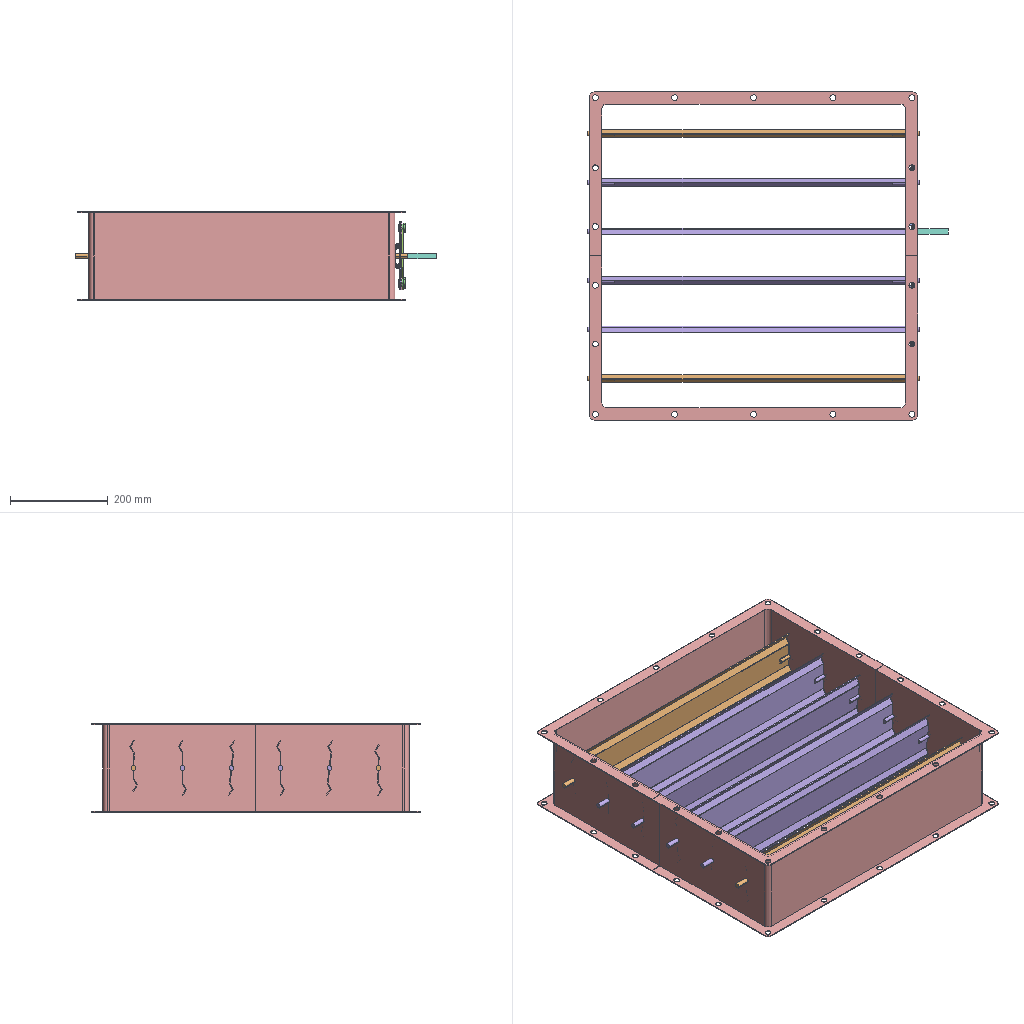Assembly | SolidWorks | 13 different items | 29 placed | box 737 x 670 x 180 mm
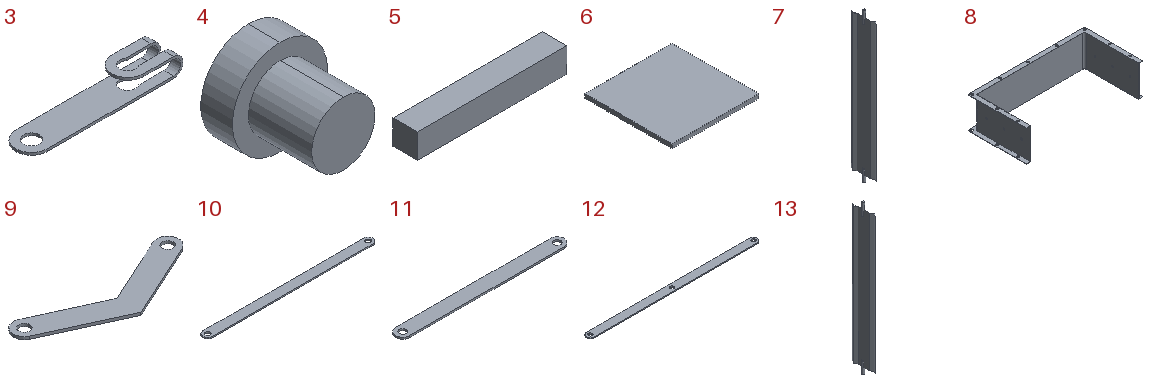Parts list (item | name | quantity | size | volume | features):
1 | B28000080  1 Type Hex Nut   Fine Thread  M8×1.5 Stainless Steel304 GB.T 6171-2000 | x1 | - | - | -
2 | B440L008C Hex Socket Head Cap Screw M8×30(Full Thread) Stainless Steel304  GB.T 70.1 | x1 | - | - | -
3 | - | x6 | 94.5 x 20 x 12 mm | 2986 mm3 | features Extrusion 1, Fillet 1, ICE 1
4 | - | x6 | 15 x 15 x 15 mm | 1669 mm3 | features Extrusion 1, ICE 1
5 | - | x1 | 75 x 12 x 12 mm | 10551 mm3 | features Extrusion 1, ICE 1
6 | - | x1 | 32 x 32 x 1.5 mm | 1536 mm3 | features Extrusion 1
7 | - | x4 | 16.5 x 113 x 678 mm | 119565 mm3 | features Extrusion 1, ICE 1, MirrorPattern 1
8 | - | x2 | 670 x 335 x 180 mm | 671550 mm3 | features ICE 3, Cut 1, Extrusion 1
9 | - | x1 | 151.1 x 51.002 x 2.5 mm | 7602 mm3 | features Extrusion 1
10 | - | x1 | 351.77 x 20 x 2.5 mm | 16981 mm3 | features Extrusion 1
11 | - | x1 | 240 x 20 x 2.5 mm | 11393 mm3 | features Extrusion 1
12 | - | x2 | 440 x 20 x 2.5 mm | 21196 mm3 | features Extrusion 1
13 | - | x2 | 16.5 x 104 x 678 mm | 111195 mm3 | features Extrusion 1, ICE 1, MirrorPattern 1
Mates (type | each side: item.copy, entity, surface, feature):
Coincident | 8.1 plane | assembly plane | 3 times
Coincident | 8.1 face plane Boss-Extrude1 | 8.2 face plane Boss-Extrude1 | 2 times
Coincident | 8.1 face plane Boss-Extrude2 | 8.2 face plane Boss-Extrude2
Coincident | 9.1 face plane Boss-Extrude1 | 12.1 face plane Boss-Extrude1
Concentric | 3.1 edge | 12.2 edge
Coincident | 3.1 face plane Boss-Extrude1 | 12.2 face plane Boss-Extrude1
Coincident | 8.1 face plane Boss-Extrude2 | 3.1 face plane Boss-Extrude1
Concentric | 9.1 edge | 12.1 edge
Concentric | 9.1 face cylinder Boss-Extrude1 | 12.2 face cylinder Boss-Extrude1
Concentric | 8.1 face cylinder Cut-Extrude2 | 5.1 face cylinder Cut-Extrude1
Parallel | 8.1 face plane Boss-Extrude1 | 5.1 face plane Boss-Extrude1
Concentric | 3.2 edge | 9.1 face cylinder Boss-Extrude1
Coincident | 3.1 face plane Boss-Extrude1 | 3.2 face plane Boss-Extrude1
Coincident | 3.2 face plane Boss-Extrude1 | 3.3 face plane Boss-Extrude1
Coincident | 3.2 face plane Boss-Extrude1 | 3.4 face plane Boss-Extrude1
Concentric | 8.2 face cylinder Cut-Extrude2 | 3.5 edge
Coincident | 3.4 face plane Boss-Extrude1 | 3.5 face plane Boss-Extrude1
Concentric | 3.5 face cylinder Cut-Extrude1 | 12.2 face cylinder Boss-Extrude1
Concentric | 3.6 edge | 12.1 face cylinder Boss-Extrude1
Concentric | 8.2 face cylinder Cut-Extrude2 | 3.6 face cylinder Cut-Extrude1
Coincident | 3.5 face plane Boss-Extrude1 | 3.6 face plane Boss-Extrude1
Coincident | 3.6 face plane Boss-Extrude1 | 12.1 face plane Boss-Extrude1
Coincident | 3.3 face plane Boss-Extrude1 | 5.1 face plane Cut-Extrude1
Concentric | 8.2 edge | 3.4 edge
Concentric | 8.1 face cylinder Cut-Extrude2 | 3.3 face cylinder Cut-Extrude1
Concentric | 8.1 edge | 3.2 edge
Concentric | 9.1 face cylinder Boss-Extrude1 | 4.1 face cylinder Boss-Extrude1
Coincident | 9.1 face plane Boss-Extrude1 | 4.1 face plane Boss-Extrude2
Concentric | 12.1 face cylinder Boss-Extrude1 | 4.2 face cylinder Boss-Extrude1
Coincident | 4.1 face plane Boss-Extrude2 | 4.2 face plane Boss-Extrude2
Concentric | 12.2 edge | 4.3 face cylinder Boss-Extrude1
Concentric | 12.1 edge | 4.4 face cylinder Boss-Extrude1
Concentric | 12.2 edge | 4.5 face cylinder Boss-Extrude1
Coincident | 12.1 edge | 4.6 face cylinder Boss-Extrude1
Coincident | 4.5 edge | 4.6 face plane Boss-Extrude2
Coincident | 4.4 face plane Boss-Extrude2 | 4.5 face plane Boss-Extrude2
Coincident | 4.3 face plane Boss-Extrude2 | 4.4 face plane Boss-Extrude2
Coincident | 4.2 face plane Boss-Extrude2 | 4.3 face plane Boss-Extrude2
Concentric | 8.2 face cylinder Cut-Extrude2 | 13.1 face cylinder Mirror1
Coincident | 3.2 edge | 7.1 face cylinder Mirror1
Concentric | 3.1 edge | 13.2 face cylinder Mirror1
Symmetric | 8.1 face plane Boss-Extrude2 | 8.1 face plane Boss-Extrude2 | 13.2 plane
Coincident | 13.2 face plane Mirror1 | 7.1 face plane Mirror1
Coincident | 13.1 face plane Mirror1 | assembly face
Concentric | 8.1 edge | 13.2 face cylinder Boss-Extrude2
Concentric | 3.3 edge | 7.2 face cylinder Mirror1
Coincident | 7.1 face plane Boss-Extrude1 | 7.2 face plane Boss-Extrude1